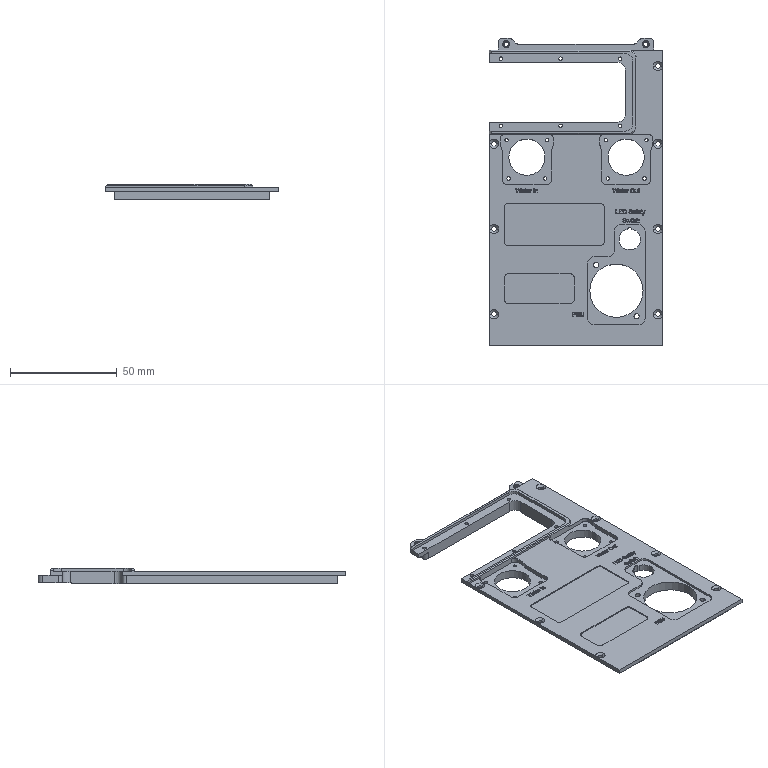Part | 1 solid | 804 faces | box 81.5 x 144.28 x 7.5 mm | volume 29990 mm3 | plane 408 | cylinder 312 | spline 64 | cone 20 | commonest cylinder face diameters 4 x56 1.6 x28 2.4 x14 2 x13 6 x6 1.738 x5